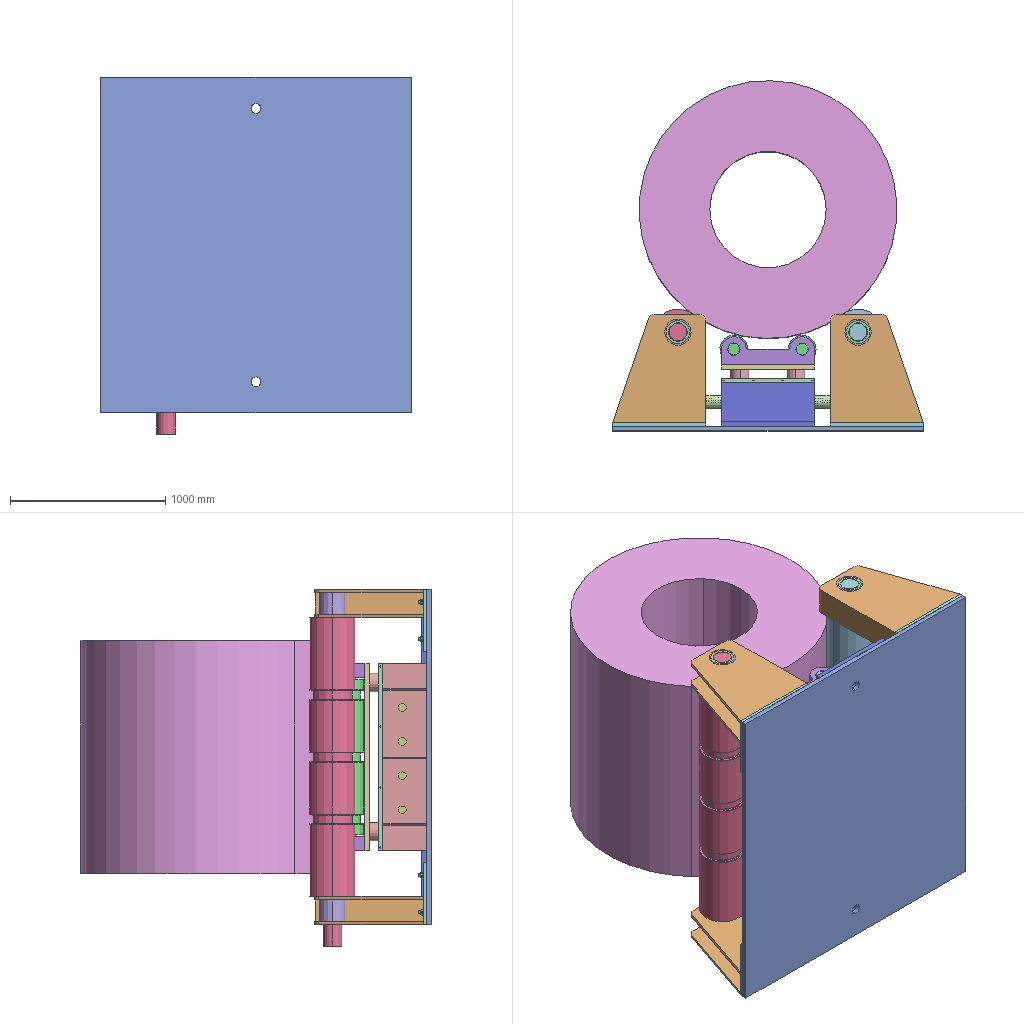Assembly | SolidWorks | 31 different items | 151 placed | box 2000 x 2255 x 2300 mm
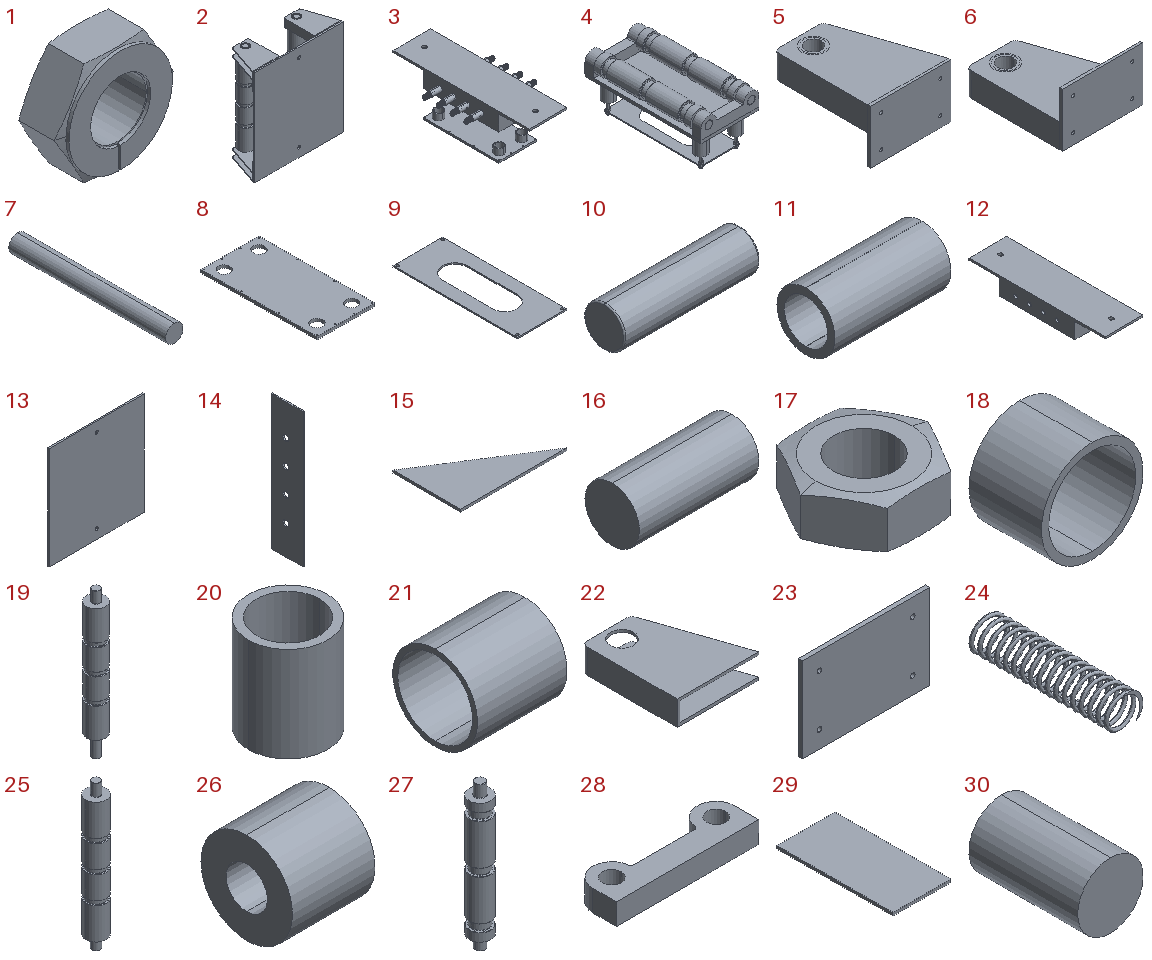Parts list (item | name | quantity | parent item | size | volume | features):
1 | (subassembly) | x16 | in 2 | 41.569 x 16.1 x 36 mm | 12517 mm3 | -
2 | (subassembly) | x1 | - | 2000 x 785 x 2300 mm | 484655330 mm3 | features ReferencePattern 23, MirrorCompFeat 5, LocalLPattern 1
3 | (subassembly) | x1 | - | 1100 x 2160 x 708.763 mm | 96729092 mm3 | features ReferencePattern 25, LocalLPattern 7, MirrorCompFeat 1, RefAxis 1
4 | (subassembly) | x1 | - | 620 x 1200 x 558 mm | 95599364 mm3 | features ReferencePattern 7, LocalLPattern 2, CompositeCurve 1
5 | (subassembly) | x2 | in 2 | 600 x 720 x 400 mm | 21248594 mm3 | -
6 | (subassembly) | x2 | in 2 | 600 x 720 x 400 mm | 21248594 mm3 | -
7 | - | x4 | in 4 | 20 x 180 x 20 mm | 56549 mm3 | features Extrusion 1
8 | - | x1 | in 3 | 600 x 1200 x 30 mm | 20172146 mm3 | features LPattern 8, ICE 3, Extrusion 1
9 | - | x1 | in 4 | 400 x 1000 x 10 mm | 2873274 mm3 | features ICE 2, Extrusion 1
10 | - | x8 | in 3 | 200 x 60 x 60 mm | 565168 mm3 | features Extrusion 1, Fillet 1
11 | - | x16 | in 3 | 160 x 80 x 80 mm | 351858 mm3 | features Extrusion 1
12 | - | x1 | in 3 | 600 x 2160 x 280 mm | 64089547 mm3 | features ICE 6, LPattern 5, Extrusion 1
13 | - | x1 | in 2 | 2000 x 80 x 2160 mm | 129658308 mm3 | features ICE 2, Extrusion 1
14 | - | x2 | in 2 | 10 x 280 x 1200 mm | 3281460 mm3 | features Extrusion 1, ICE 1, LPattern 1
15 | - | x6 | in 2 | 440 x 280 x 10 mm | 616000 mm3 | features Extrusion 1
16 | - | x8 | in 2 | 110 x 50 x 50 mm | 215984 mm3 | features Extrusion 1
17 | - | x24 | in 1, 4 | 41.569 x 36 x 15 mm | 11785 mm3 | features Extrusion 1, RevCut 1
18 | - | x4 | in 3 | 140 x 100 x 140 mm | 408407 mm3 | features Extrusion 1
19 | - | x1 | in 2 | 300 x 300 x 2300 mm | 129677535 mm3 | features ICE 3, Chamfer 2, Extrusion 1, Fillet 1, LPattern 1, RefAxis 1, RevCut 1
20 | - | x4 | in 5, 6 | 150 x 150 x 180 mm | 1145111 mm3 | features Extrusion 1
21 | - | x4 | in 5, 6 | 180 x 170 x 170 mm | 904779 mm3 | features Extrusion 1
22 | - | x4 | in 5, 6 | 600 x 700 x 180 mm | 14429116 mm3 | features ICE 3, Fillet 2, Extrusion 1
23 | - | x4 | in 5, 6 | 600 x 20 x 400 mm | 4769589 mm3 | features Extrusion 1, ICE 1
24 | - | x8 | in 3 | 62 x 250 x 62 mm | 81996 mm3 | features Helix 1, ICE 1, RefAxis 1, Sweep 1
25 | - | x1 | in 2 | 300 x 300 x 2160 mm | 128138036 mm3 | features Chamfer 2, ICE 2, Extrusion 1, Fillet 1, LPattern 1, RefAxis 1, RevCut 1
26 | - | x1 | - | 1500 x 1660 x 1660 mm | 2583685068 mm3 | features Extrusion 1
27 | - | x2 | in 4 | 180 x 180 x 1200 mm | 24641407 mm3 | features Chamfer 2, ICE 2, Extrusion 1, Fillet 1, LPattern 1, RefAxis 1, RevCut 1
28 | - | x2 | in 4 | 600 x 180 x 90 mm | 6307881 mm3 | features Extrusion 1
29 | - | x1 | in 4 | 600 x 1200 x 30 mm | 21509522 mm3 | features Extrusion 1, ICE 1
30 | - | x4 | in 4 | 120 x 200 x 120 mm | 2249380 mm3 | features Extrusion 1, ICE 1
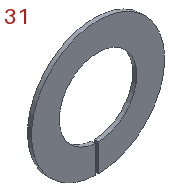31 | - | x16 | in 1 | 36 x 1.1 x 36 mm | 732.535 mm3 | features Extrusion 1
Mates (type | each side: item.copy, entity, surface, feature):
In the top assembly
Coincident | 13.1 face plane Boss-Extrude1 | 12.1 face plane Boss-Extrude1
Concentric | 13.1 face cylinder Cut-Extrude1 | 12.1 face cylinder Cut-Extrude4 | 2 times
Concentric | 18.1 face cylinder Boss-Extrude1 | 30.1 face cylinder Boss-Extrude2
Concentric | 18.2 face cylinder Boss-Extrude1 | 30.2 face cylinder Boss-Extrude2
DistanceDim | 26.1 face plane Boss-Extrude1 | 22.1 face plane Boss-Extrude1
Tangent | 25.1 face cylinder Boss-Extrude1 | 26.1 face cylinder Boss-Extrude1
Tangent | 19.1 face cylinder Boss-Extrude1 | 26.1 face cylinder Boss-Extrude1
In subassembly 2
Coincident | 14.1 face plane Boss-Extrude1 | 13.2 face plane Boss-Extrude1
DistanceDim | 14.1 face plane Boss-Extrude1 | 13.2 face plane Boss-Extrude1
Concentric | 14.1 face cylinder LPattern1 | 16.1 face cylinder Boss-Extrude1
Coincident | 14.1 face plane Boss-Extrude1 | 16.1 face plane Boss-Extrude1
DistanceDim | 14.2 face plane Boss-Extrude1 | 13.2 face plane Boss-Extrude1
Coincident | 13.2 face plane Boss-Extrude1 | 15.1 face plane Boss-Extrude1
Coincident | 14.1 face plane Boss-Extrude1 | 15.1 face plane Boss-Extrude1
DistanceDim | 15.1 face plane Boss-Extrude1 | 14.1 face plane Boss-Extrude1
Coincident | 13.2 face plane Boss-Extrude1 | 15.2 face plane Boss-Extrude1
Coincident | 14.1 face plane Boss-Extrude1 | 15.2 face plane Boss-Extrude1
DistanceDim | 15.2 face plane Boss-Extrude1 | 14.1 face plane Boss-Extrude1
Coincident | 13.2 face plane Boss-Extrude1 | 15.3 face plane Boss-Extrude1
Coincident | 14.1 face plane Boss-Extrude1 | 15.3 face plane Boss-Extrude1
DistanceDim | 15.3 face plane Boss-Extrude1 | 15.1 face plane Boss-Extrude1
Coincident | 13.2 face plane Boss-Extrude1 | 23.1 face plane Boss-Extrude1 | 3 times
Coincident | 13.2 face plane Boss-Extrude1 | 23.2 face plane Boss-Extrude1 | 3 times
Coincident | 13.2 face plane Boss-Extrude1 | 23.3 face plane Boss-Extrude1 | 2 times
Coincident | 13.2 face plane Boss-Extrude1 | 22.2 face plane Boss-Extrude1
Coincident | 13.2 face plane Boss-Extrude1 | 23.4 face plane Boss-Extrude1 | 2 times
Coincident | 13.2 face plane Boss-Extrude1 | 22.3 face plane Boss-Extrude1
Coincident | 22.3 face plane Boss-Extrude1 | 19.2 face plane Boss-Extrude2
Concentric | 20.1 face cylinder Boss-Extrude1 | 19.2 face cylinder Boss-Extrude2
Coincident | 22.4 face plane Boss-Extrude1 | 25.2 face plane Boss-Extrude3
Concentric | 20.2 face cylinder Boss-Extrude1 | 25.2 face cylinder Boss-Extrude3
Coincident | 23.4 face plane Boss-Extrude1 | 31.1 face plane Boss-Extrude1
Concentric | 13.2 face cylinder Boss-Extrude2 | 17.1 face cylinder Boss-Extrude1
Coincident | 23.4 face plane Boss-Extrude1 | 31.2 face plane Boss-Extrude1
Concentric | 13.2 face cylinder Boss-Extrude2 | 17.2 face cylinder Boss-Extrude1
Coincident | 23.4 face plane Boss-Extrude1 | 31.3 face plane Boss-Extrude1
Concentric | 13.2 face cylinder Boss-Extrude2 | 17.3 face cylinder Boss-Extrude1
Coincident | 23.4 face plane Boss-Extrude1 | 31.4 face plane Boss-Extrude1
Concentric | 13.2 face cylinder Boss-Extrude2 | 17.4 face cylinder Boss-Extrude1
In subassembly 1
Coincident | 31.5 face plane Boss-Extrude1 | 17.5 face plane Boss-Extrude1
Concentric | 31.5 face cylinder Boss-Extrude1 | 17.5 face cylinder Boss-Extrude1
In subassembly 6
Coincident | 23.5 face plane Boss-Extrude1 | 22.5 face plane Boss-Extrude1 | 3 times
Concentric | 22.5 face cylinder Cut-Extrude1 | 21.1 face cylinder Boss-Extrude1
Coincident | 22.5 face plane Boss-Extrude1 | 21.1 face plane Boss-Extrude1
Concentric | 21.1 face cylinder Boss-Extrude1 | 20.3 face cylinder Boss-Extrude1
Coincident | 22.5 face plane Boss-Extrude1 | 20.3 face plane Boss-Extrude1
In subassembly 5
Coincident | 23.5 face plane Boss-Extrude1 | 22.5 face plane Boss-Extrude1 | 3 times
Concentric | 22.5 face cylinder Cut-Extrude1 | 21.1 face cylinder Boss-Extrude1
Coincident | 22.5 face plane Boss-Extrude1 | 21.1 face plane Boss-Extrude1
Concentric | 21.1 face cylinder Boss-Extrude1 | 20.3 face cylinder Boss-Extrude1
Coincident | 22.5 face plane Boss-Extrude1 | 20.3 face plane Boss-Extrude1
In subassembly 4
Coincident | 29.1 face plane Boss-Extrude1 | 28.1 face plane Boss-Extrude2 | 3 times
Concentric | 28.1 face cylinder Boss-Extrude2 | 27.1 face cylinder Boss-Extrude2 | 2 times
Coincident | 28.1 face plane Boss-Extrude2 | 27.1 face plane Boss-Extrude2
Coincident | 29.1 face plane Boss-Extrude1 | 28.2 face plane Boss-Extrude2 | 2 times
Concentric | 27.1 face cylinder Boss-Extrude3 | 28.2 face cylinder Boss-Extrude2
Concentric | 28.1 face cylinder Boss-Extrude2 | 27.2 face cylinder Boss-Extrude2
Coincident | 28.1 face plane Boss-Extrude2 | 27.2 face plane Boss-Extrude2
Coincident | 29.1 face plane Cut-Extrude1 | 30.3 face plane Boss-Extrude2
Concentric | 29.1 face cylinder Cut-Extrude1 | 30.3 face cylinder Boss-Extrude2
Coincident | 29.1 face plane Cut-Extrude1 | 30.4 face plane Boss-Extrude2
Coincident | 29.1 edge | 30.4 face cylinder Boss-Extrude2
Coincident | 29.1 face plane Cut-Extrude1 | 30.5 face plane Boss-Extrude2
Concentric | 29.1 face cylinder Cut-Extrude1 | 30.5 face cylinder Boss-Extrude2
Coincident | 29.1 face plane Cut-Extrude1 | 30.6 face plane Boss-Extrude2
Concentric | 29.1 face cylinder Cut-Extrude1 | 30.6 face cylinder Boss-Extrude2
Coincident | 30.6 face plane Cut-Extrude2 | 7.1 face plane Boss-Extrude1
Concentric | 30.6 face cylinder Cut-Extrude2 | 7.1 face cylinder Boss-Extrude1
Coincident | 30.5 face plane Cut-Extrude2 | 7.2 face plane Boss-Extrude1
Concentric | 30.5 face cylinder Cut-Extrude2 | 7.2 face cylinder Boss-Extrude1
Coincident | 30.4 face plane Cut-Extrude2 | 7.3 face plane Boss-Extrude1
Concentric | 30.4 face cylinder Cut-Extrude2 | 7.3 face cylinder Boss-Extrude1
Coincident | 30.3 face plane Cut-Extrude2 | 7.4 face plane Boss-Extrude1
Concentric | 30.3 face cylinder Cut-Extrude2 | 7.4 face cylinder Boss-Extrude1
Concentric | 7.4 face cylinder Boss-Extrude1 | 17.5 face cylinder Boss-Extrude1
DistanceDim | 17.5 face plane Boss-Extrude1 | 7.4 face plane Boss-Extrude1
Coincident | 17.6 face plane Boss-Extrude1 | 9.1 face plane Boss-Extrude1
Concentric | 7.1 face cylinder Boss-Extrude1 | 9.1 face cylinder Cut-Extrude1
Concentric | 7.3 face cylinder Boss-Extrude1 | 9.1 face cylinder Cut-Extrude1
In subassembly 3
Concentric | 8.1 face cylinder Cut-Extrude1 | 18.3 face cylinder Boss-Extrude1
Concentric | 8.1 face cylinder Cut-Extrude1 | 18.4 face cylinder Boss-Extrude1
Concentric | 8.1 face cylinder Cut-Extrude1 | 18.5 face cylinder Boss-Extrude1
Concentric | 8.1 face cylinder Cut-Extrude1 | 18.6 face cylinder Boss-Extrude1
Coincident | 12.2 face plane Boss-Extrude2 | 11.1 face plane Boss-Extrude1
Concentric | 12.2 face cylinder LPattern1 | 11.1 face cylinder Boss-Extrude1
Coincident | 12.2 face plane Boss-Extrude2 | 11.2 face plane Boss-Extrude1
Concentric | 12.2 face cylinder LPattern1 | 11.2 face cylinder Boss-Extrude1
Coincident | 8.1 face plane Boss-Extrude1 | 12.2 face plane Boss-Extrude1 | 2 times
Coincident | 8.1 face plane Boss-Extrude1 | 12.2 face plane Boss-Extrude2
Coincident | 12.2 face plane Boss-Extrude1 | 11.3 face plane Boss-Extrude1
Concentric | 12.2 face cylinder LPattern1 | 11.3 face cylinder Boss-Extrude1
Coincident | 12.2 face plane Boss-Extrude1 | 11.4 face plane Boss-Extrude1
Concentric | 12.2 face cylinder Cut-Extrude2 | 11.4 face cylinder Boss-Extrude1
Concentric | 11.3 face cylinder Boss-Extrude1 | 10.1 face cylinder Boss-Extrude1
Coincident | 12.2 face plane Boss-Extrude1 | 10.1 face plane Boss-Extrude1
Concentric | 11.5 face cylinder Boss-Extrude1 | 10.2 face cylinder Boss-Extrude1
Coincident | 12.2 face plane Boss-Extrude1 | 10.2 face plane Boss-Extrude1
Coincident | 10.1 face plane Boss-Extrude1 | 24.1 face plane Cut-Extrude1
Coincident | 24.1 axis | 3.1 axis